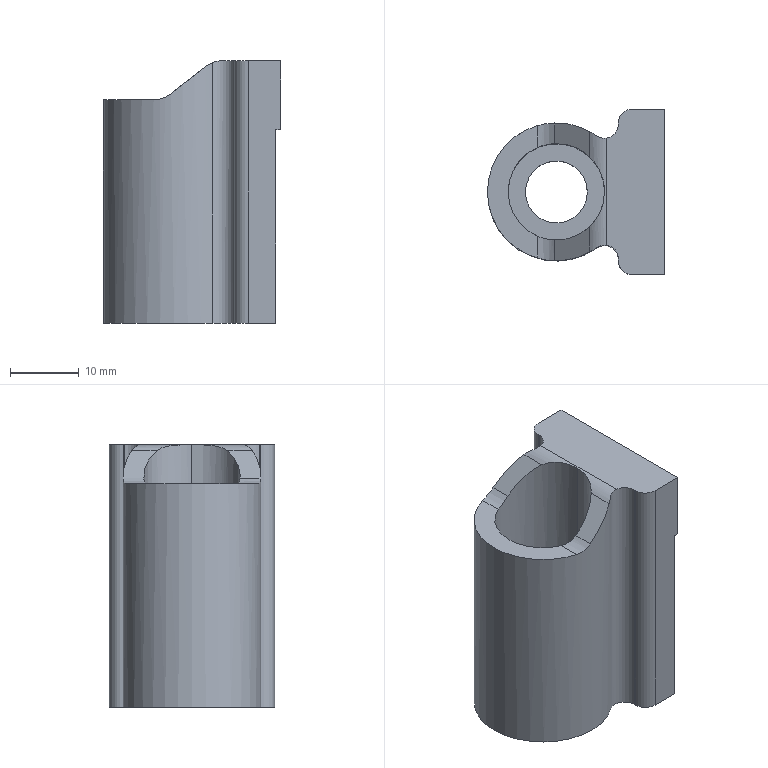Part | STEP file | 1_id1170_x_t | 1 solid | 25 faces | box 25.7 x 24 x 38.1 mm | volume 13011 mm3 | plane 13 | cylinder 12 | commonest cylinder face diameters 4 x4 8 x3 9 x2 14 x2 20 x1